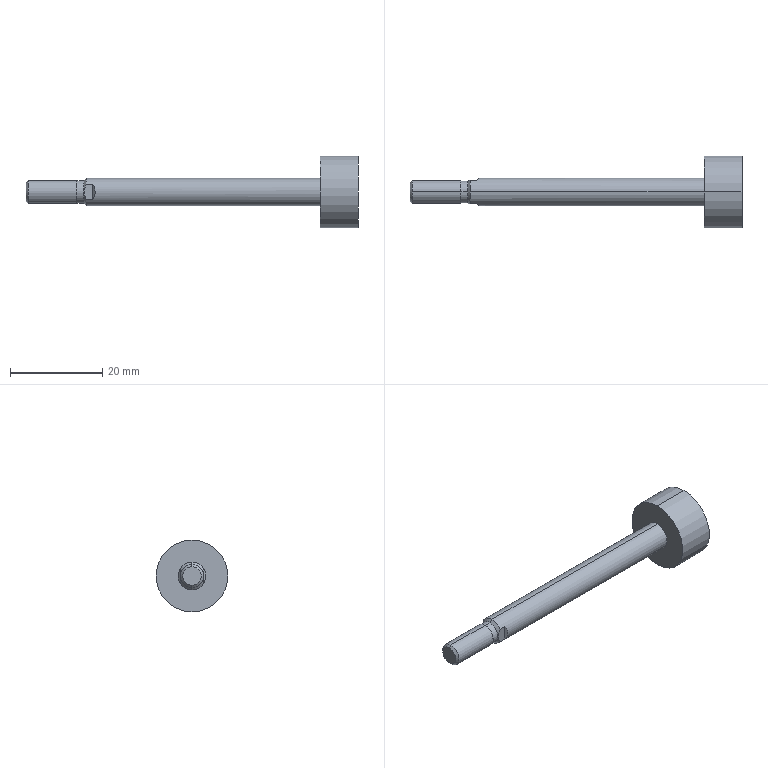Part | SolidWorks | features BaseBody 1 | 1 solid | 20 faces | box 72 x 15.6 x 15.6 mm | volume 3252 mm3 | plane 8 | cylinder 8 | cone 4 | commonest cylinder face diameters 4.8 x2 5 x2 6 x2 15.6 x2
STEP:
#1=CARTESIAN_POINT('',(-16.,0.,-2.01));
#2=VERTEX_POINT('',#1);
#3=CARTESIAN_POINT('',(-16.,0.,2.01));
#4=VERTEX_POINT('',#3);
#5=CARTESIAN_POINT('',(-16.,0.,0.));
#6=DIRECTION('',(1.,0.,0.));
#7=DIRECTION('',(0.,0.,-1.));
#8=AXIS2_PLACEMENT_3D('',#5,#6,#7);
#9=CIRCLE('',#8,2.01);
#10=EDGE_CURVE('',#2,#4,#9,.T.);
#11=ORIENTED_EDGE('',*,*,#10,.F.);
#12=CARTESIAN_POINT('',(-16.,0.,0.));
#13=DIRECTION('',(1.,0.,0.));
#14=DIRECTION('',(0.,0.,-1.));
#15=AXIS2_PLACEMENT_3D('',#12,#13,#14);
#16=CIRCLE('',#15,2.01);
#17=EDGE_CURVE('',#4,#2,#16,.T.);
#18=ORIENTED_EDGE('',*,*,#17,.F.);
#19=EDGE_LOOP('',(#11,#18));
#20=FACE_OUTER_BOUND('',#19,.T.);
#21=CARTESIAN_POINT('',(-16.,0.,0.));
#22=DIRECTION('',(1.,0.,0.));
#23=DIRECTION('',(0.,1.,0.));
#24=AXIS2_PLACEMENT_3D('',#21,#22,#23);
#25=PLANE('',#24);
#26=ADVANCED_FACE('',(#20),#25,.F.);
#27=CARTESIAN_POINT('',(-15.51,0.,2.5));
#28=VERTEX_POINT('',#27);
#29=CARTESIAN_POINT('',(-15.51,0.,2.5));
#30=DIRECTION('',(0.7071,0.,0.7071));
#31=VECTOR('',#30,1000.);
#32=LINE('',#29,#31);
#33=EDGE_CURVE('',#4,#28,#32,.T.);
#34=ORIENTED_EDGE('',*,*,#33,.F.);
#35=ORIENTED_EDGE('',*,*,#17,.T.);
#36=CARTESIAN_POINT('',(-15.51,0.,-2.5));
#37=VERTEX_POINT('',#36);
#38=CARTESIAN_POINT('',(-15.51,0.,-2.5));
#39=DIRECTION('',(0.7071,0.,-0.7071));
#40=VECTOR('',#39,1000.);
#41=LINE('',#38,#40);
#42=EDGE_CURVE('',#2,#37,#41,.T.);
#43=ORIENTED_EDGE('',*,*,#42,.T.);
#44=CARTESIAN_POINT('',(-15.51,0.,0.));
#45=DIRECTION('',(1.,0.,0.));
#46=DIRECTION('',(0.,0.,1.));
#47=AXIS2_PLACEMENT_3D('',#44,#45,#46);
#48=CIRCLE('',#47,2.5);
#49=EDGE_CURVE('',#28,#37,#48,.T.);
#50=ORIENTED_EDGE('',*,*,#49,.F.);
#51=EDGE_LOOP('',(#34,#35,#43,#50));
#52=FACE_OUTER_BOUND('',#51,.T.);
#53=CARTESIAN_POINT('',(-15.51,0.,0.));
#54=DIRECTION('',(1.,0.,0.));
#55=DIRECTION('',(0.,0.,-1.));
#56=AXIS2_PLACEMENT_3D('',#53,#54,#55);
#57=CONICAL_SURFACE('',#56,2.5,0.7854);
#58=ADVANCED_FACE('',(#52),#57,.T.);
#59=CARTESIAN_POINT('',(-5.,0.,-2.5));
#60=VERTEX_POINT('',#59);
#61=CARTESIAN_POINT('',(56.,0.,-2.5));
#62=DIRECTION('',(-1.,0.,0.));
#63=VECTOR('',#62,1000.);
#64=LINE('',#61,#63);
#65=EDGE_CURVE('',#60,#37,#64,.T.);
#66=ORIENTED_EDGE('',*,*,#65,.F.);
#67=CARTESIAN_POINT('',(-5.,0.,2.5));
#68=VERTEX_POINT('',#67);
#69=CARTESIAN_POINT('',(-5.,0.,0.));
#70=DIRECTION('',(-1.,0.,0.));
#71=DIRECTION('',(0.,0.,1.));
#72=AXIS2_PLACEMENT_3D('',#69,#70,#71);
#73=CIRCLE('',#72,2.5);
#74=EDGE_CURVE('',#60,#68,#73,.T.);
#75=ORIENTED_EDGE('',*,*,#74,.T.);
#76=CARTESIAN_POINT('',(56.,0.,2.5));
#77=DIRECTION('',(-1.,0.,0.));
#78=VECTOR('',#77,1000.);
#79=LINE('',#76,#78);
#80=EDGE_CURVE('',#68,#28,#79,.T.);
#81=ORIENTED_EDGE('',*,*,#80,.T.);
#82=ORIENTED_EDGE('',*,*,#49,.T.);
#83=EDGE_LOOP('',(#66,#75,#81,#82));
#84=FACE_OUTER_BOUND('',#83,.T.);
#85=CARTESIAN_POINT('',(56.,0.,0.));
#86=DIRECTION('',(-1.,0.,0.));
#87=DIRECTION('',(0.,0.,1.));
#88=AXIS2_PLACEMENT_3D('',#85,#86,#87);
#89=CYLINDRICAL_SURFACE('',#88,2.5);
#90=ADVANCED_FACE('',(#84),#89,.T.);
#91=CARTESIAN_POINT('',(56.,0.,7.8));
#92=VERTEX_POINT('',#91);
#93=CARTESIAN_POINT('',(56.,0.,-7.8));
#94=VERTEX_POINT('',#93);
#95=CARTESIAN_POINT('',(56.,0.,0.));
#96=DIRECTION('',(-1.,0.,0.));
#97=DIRECTION('',(0.,0.,1.));
#98=AXIS2_PLACEMENT_3D('',#95,#96,#97);
#99=CIRCLE('',#98,7.8);
#100=EDGE_CURVE('',#92,#94,#99,.T.);
#101=ORIENTED_EDGE('',*,*,#100,.F.);
#102=CARTESIAN_POINT('',(56.,0.,0.));
#103=DIRECTION('',(-1.,0.,0.));
#104=DIRECTION('',(0.,0.,1.));
#105=AXIS2_PLACEMENT_3D('',#102,#103,#104);
#106=CIRCLE('',#105,7.8);
#107=EDGE_CURVE('',#94,#92,#106,.T.);
#108=ORIENTED_EDGE('',*,*,#107,.F.);
#109=EDGE_LOOP('',(#101,#108));
#110=FACE_OUTER_BOUND('',#109,.T.);
#111=CARTESIAN_POINT('',(56.,7.8,0.));
#112=DIRECTION('',(-1.,0.,0.));
#113=DIRECTION('',(0.,0.,1.));
#114=AXIS2_PLACEMENT_3D('',#111,#112,#113);
#115=PLANE('',#114);
#116=ADVANCED_FACE('',(#110),#115,.F.);
#117=CARTESIAN_POINT('',(-5.,0.,2.4));
#118=VERTEX_POINT('',#117);
#119=CARTESIAN_POINT('',(-5.,0.,-2.4));
#120=VERTEX_POINT('',#119);
#121=CARTESIAN_POINT('',(-5.,0.,0.));
#122=DIRECTION('',(1.,0.,0.));
#123=DIRECTION('',(0.,0.,1.));
#124=AXIS2_PLACEMENT_3D('',#121,#122,#123);
#125=CIRCLE('',#124,2.4);
#126=EDGE_CURVE('',#118,#120,#125,.T.);
#127=ORIENTED_EDGE('',*,*,#126,.F.);
#128=CARTESIAN_POINT('',(-5.,0.,0.));
#129=DIRECTION('',(1.,0.,0.));
#130=DIRECTION('',(0.,0.,1.));
#131=AXIS2_PLACEMENT_3D('',#128,#129,#130);
#132=CIRCLE('',#131,2.4);
#133=EDGE_CURVE('',#120,#118,#132,.T.);
#134=ORIENTED_EDGE('',*,*,#133,.F.);
#135=EDGE_LOOP('',(#127,#134));
#136=FACE_BOUND('',#135,.T.);
#137=CARTESIAN_POINT('',(-5.,0.,0.));
#138=DIRECTION('',(-1.,0.,0.));
#139=DIRECTION('',(0.,0.,1.));
#140=AXIS2_PLACEMENT_3D('',#137,#138,#139);
#141=CIRCLE('',#140,2.5);
#142=EDGE_CURVE('',#68,#60,#141,.T.);
#143=ORIENTED_EDGE('',*,*,#142,.F.);
#144=ORIENTED_EDGE('',*,*,#74,.F.);
#145=EDGE_LOOP('',(#143,#144));
#146=FACE_OUTER_BOUND('',#145,.T.);
#147=CARTESIAN_POINT('',(-5.,2.5,0.));
#148=DIRECTION('',(-1.,0.,0.));
#149=DIRECTION('',(0.,0.,1.));
#150=AXIS2_PLACEMENT_3D('',#147,#148,#149);
#151=PLANE('',#150);
#152=ADVANCED_FACE('',(#136,#146),#151,.F.);
#153=CARTESIAN_POINT('',(47.8,0.,-7.8));
#154=VERTEX_POINT('',#153);
#155=CARTESIAN_POINT('',(56.,0.,-7.8));
#156=DIRECTION('',(-1.,0.,0.));
#157=VECTOR('',#156,1000.);
#158=LINE('',#155,#157);
#159=EDGE_CURVE('',#94,#154,#158,.T.);
#160=ORIENTED_EDGE('',*,*,#159,.F.);
#161=ORIENTED_EDGE('',*,*,#107,.T.);
#162=CARTESIAN_POINT('',(47.8,0.,7.8));
#163=VERTEX_POINT('',#162);
#164=CARTESIAN_POINT('',(56.,0.,7.8));
#165=DIRECTION('',(-1.,0.,0.));
#166=VECTOR('',#165,1000.);
#167=LINE('',#164,#166);
#168=EDGE_CURVE('',#92,#163,#167,.T.);
#169=ORIENTED_EDGE('',*,*,#168,.T.);
#170=CARTESIAN_POINT('',(47.8,0.,0.));
#171=DIRECTION('',(1.,0.,0.));
#172=DIRECTION('',(0.,0.,1.));
#173=AXIS2_PLACEMENT_3D('',#170,#171,#172);
#174=CIRCLE('',#173,7.8);
#175=EDGE_CURVE('',#163,#154,#174,.T.);
#176=ORIENTED_EDGE('',*,*,#175,.T.);
#177=EDGE_LOOP('',(#160,#161,#169,#176));
#178=FACE_OUTER_BOUND('',#177,.T.);
#179=CARTESIAN_POINT('',(56.,0.,0.));
#180=DIRECTION('',(-1.,0.,0.));
#181=DIRECTION('',(0.,0.,1.));
#182=AXIS2_PLACEMENT_3D('',#179,#180,#181);
#183=CYLINDRICAL_SURFACE('',#182,7.8);
#184=ADVANCED_FACE('',(#178),#183,.T.);
#185=CARTESIAN_POINT('',(-1.5,2.5,-1.658));
#186=VERTEX_POINT('',#185);
#187=CARTESIAN_POINT('',(-2.9,2.5,-1.658));
#188=VERTEX_POINT('',#187);
#189=CARTESIAN_POINT('',(-18.5,2.5,-1.658));
#190=DIRECTION('',(-1.,0.,0.));
#191=VECTOR('',#190,1000.);
#192=LINE('',#189,#191);
#193=EDGE_CURVE('',#186,#188,#192,.T.);
#194=ORIENTED_EDGE('',*,*,#193,.T.);
#195=CARTESIAN_POINT('',(-2.9,2.5,1.658));
#196=VERTEX_POINT('',#195);
#197=CARTESIAN_POINT('',(-2.9,2.5,1.658));
#198=CARTESIAN_POINT('',(-2.976,2.5,1.52));
#199=CARTESIAN_POINT('',(-3.044,2.5,1.385));
#200=CARTESIAN_POINT('',(-3.133,2.5,1.187));
#201=CARTESIAN_POINT('',(-3.161,2.5,1.121));
#202=CARTESIAN_POINT('',(-3.199,2.5,1.024));
#203=CARTESIAN_POINT('',(-3.217,2.5,0.9749));
#204=CARTESIAN_POINT('',(-3.234,2.5,0.9264));
#205=CARTESIAN_POINT('',(-3.245,2.5,0.8941));
#206=CARTESIAN_POINT('',(-3.25,2.5,0.8796));
#207=CARTESIAN_POINT('',(-3.279,2.5,0.7907));
#208=CARTESIAN_POINT('',(-3.299,2.5,0.7199));
#209=CARTESIAN_POINT('',(-3.326,2.5,0.6139));
#210=CARTESIAN_POINT('',(-3.334,2.5,0.5785));
#211=CARTESIAN_POINT('',(-3.349,2.5,0.5078));
#212=CARTESIAN_POINT('',(-3.356,2.5,0.4737));
#213=CARTESIAN_POINT('',(-3.387,2.5,0.2894));
#214=CARTESIAN_POINT('',(-3.4,2.5,0.1457));
#215=CARTESIAN_POINT('',(-3.4,2.5,-0.1432));
#216=CARTESIAN_POINT('',(-3.388,2.5,-0.2845));
#217=CARTESIAN_POINT('',(-3.352,2.5,-0.4978));
#218=CARTESIAN_POINT('',(-3.337,2.5,-0.5692));
#219=CARTESIAN_POINT('',(-3.31,2.5,-0.6771));
#220=CARTESIAN_POINT('',(-3.296,2.5,-0.7314));
#221=CARTESIAN_POINT('',(-3.277,2.5,-0.7952));
#222=CARTESIAN_POINT('',(-3.268,2.5,-0.8227));
#223=CARTESIAN_POINT('',(-3.262,2.5,-0.8411));
#224=CARTESIAN_POINT('',(-3.259,2.5,-0.8514));
#225=CARTESIAN_POINT('',(-3.172,2.5,-1.118));
#226=CARTESIAN_POINT('',(-3.053,2.5,-1.381));
#227=CARTESIAN_POINT('',(-2.9,2.5,-1.658));
#228=B_SPLINE_CURVE_WITH_KNOTS('',3,(#197,#198,#199,#200,#201,#202,#203,#204,#205,#206,#207,#208,#209,#210,#211,#212,#213,#214,#215,#216,#217,#218,#219,#220,#221,#222,#223,#224,#225,#226,#227),.UNSPECIFIED.,.F.,.F.,(4,2,2,1,2,2,2,2,2,2,2,2,1,1,2,2,4),(0.,0.125,0.1875,0.2187,0.2344,0.25,0.3125,0.3437,0.375,0.5,0.625,0.6875,0.7187,0.7344,0.7422,0.75,1.),.UNSPECIFIED.);
#229=EDGE_CURVE('',#196,#188,#228,.T.);
#230=ORIENTED_EDGE('',*,*,#229,.F.);
#231=CARTESIAN_POINT('',(-1.5,2.5,1.658));
#232=VERTEX_POINT('',#231);
#233=CARTESIAN_POINT('',(-18.5,2.5,1.658));
#234=DIRECTION('',(1.,0.,0.));
#235=VECTOR('',#234,1000.);
#236=LINE('',#233,#235);
#237=EDGE_CURVE('',#196,#232,#236,.T.);
#238=ORIENTED_EDGE('',*,*,#237,.T.);
#239=CARTESIAN_POINT('',(-1.5,2.5,6.));
#240=DIRECTION('',(0.,0.,1.));
#241=VECTOR('',#240,1000.);
#242=LINE('',#239,#241);
#243=EDGE_CURVE('',#186,#232,#242,.T.);
#244=ORIENTED_EDGE('',*,*,#243,.F.);
#245=EDGE_LOOP('',(#194,#230,#238,#244));
#246=FACE_OUTER_BOUND('',#245,.T.);
#247=CARTESIAN_POINT('',(-18.5,2.5,6.));
#248=DIRECTION('',(0.,1.,0.));
#249=DIRECTION('',(1.,0.,0.));
#250=AXIS2_PLACEMENT_3D('',#247,#248,#249);
#251=PLANE('',#250);
#252=ADVANCED_FACE('',(#246),#251,.T.);
#253=CARTESIAN_POINT('',(-1.5,-2.5,1.658));
#254=VERTEX_POINT('',#253);
#255=CARTESIAN_POINT('',(-2.9,-2.5,1.658));
#256=VERTEX_POINT('',#255);
#257=CARTESIAN_POINT('',(-1.5,-2.5,1.658));
#258=DIRECTION('',(-1.,0.,0.));
#259=VECTOR('',#258,1000.);
#260=LINE('',#257,#259);
#261=EDGE_CURVE('',#254,#256,#260,.T.);
#262=ORIENTED_EDGE('',*,*,#261,.T.);
#263=CARTESIAN_POINT('',(-2.9,-2.5,-1.658));
#264=VERTEX_POINT('',#263);
#265=CARTESIAN_POINT('',(-2.9,-2.5,-1.658));
#266=CARTESIAN_POINT('',(-2.976,-2.5,-1.52));
#267=CARTESIAN_POINT('',(-3.044,-2.5,-1.385));
#268=CARTESIAN_POINT('',(-3.133,-2.5,-1.187));
#269=CARTESIAN_POINT('',(-3.161,-2.5,-1.121));
#270=CARTESIAN_POINT('',(-3.199,-2.5,-1.024));
#271=CARTESIAN_POINT('',(-3.217,-2.5,-0.9749));
#272=CARTESIAN_POINT('',(-3.234,-2.5,-0.9264));
#273=CARTESIAN_POINT('',(-3.245,-2.5,-0.8941));
#274=CARTESIAN_POINT('',(-3.25,-2.5,-0.8796));
#275=CARTESIAN_POINT('',(-3.279,-2.5,-0.7907));
#276=CARTESIAN_POINT('',(-3.299,-2.5,-0.7199));
#277=CARTESIAN_POINT('',(-3.326,-2.5,-0.6139));
#278=CARTESIAN_POINT('',(-3.334,-2.5,-0.5785));
#279=CARTESIAN_POINT('',(-3.349,-2.5,-0.5078));
#280=CARTESIAN_POINT('',(-3.356,-2.5,-0.4737));
#281=CARTESIAN_POINT('',(-3.387,-2.5,-0.2894));
#282=CARTESIAN_POINT('',(-3.4,-2.5,-0.1457));
#283=CARTESIAN_POINT('',(-3.4,-2.5,0.1432));
#284=CARTESIAN_POINT('',(-3.388,-2.5,0.2845));
#285=CARTESIAN_POINT('',(-3.352,-2.5,0.4978));
#286=CARTESIAN_POINT('',(-3.337,-2.5,0.5692));
#287=CARTESIAN_POINT('',(-3.31,-2.5,0.6771));
#288=CARTESIAN_POINT('',(-3.296,-2.5,0.7314));
#289=CARTESIAN_POINT('',(-3.277,-2.5,0.7952));
#290=CARTESIAN_POINT('',(-3.268,-2.5,0.8227));
#291=CARTESIAN_POINT('',(-3.262,-2.5,0.8411));
#292=CARTESIAN_POINT('',(-3.259,-2.5,0.8514));
#293=CARTESIAN_POINT('',(-3.172,-2.5,1.118));
#294=CARTESIAN_POINT('',(-3.053,-2.5,1.381));
#295=CARTESIAN_POINT('',(-2.9,-2.5,1.658));
#296=B_SPLINE_CURVE_WITH_KNOTS('',3,(#265,#266,#267,#268,#269,#270,#271,#272,#273,#274,#275,#276,#277,#278,#279,#280,#281,#282,#283,#284,#285,#286,#287,#288,#289,#290,#291,#292,#293,#294,#295),.UNSPECIFIED.,.F.,.F.,(4,2,2,1,2,2,2,2,2,2,2,2,1,1,2,2,4),(0.,0.125,0.1875,0.2187,0.2344,0.25,0.3125,0.3438,0.375,0.5,0.625,0.6875,0.7188,0.7344,0.7422,0.75,1.),.UNSPECIFIED.);
#297=EDGE_CURVE('',#264,#256,#296,.T.);
#298=ORIENTED_EDGE('',*,*,#297,.F.);
#299=CARTESIAN_POINT('',(-1.5,-2.5,-1.658));
#300=VERTEX_POINT('',#299);
#301=CARTESIAN_POINT('',(-1.5,-2.5,-1.658));
#302=DIRECTION('',(1.,0.,0.));
#303=VECTOR('',#302,1000.);
#304=LINE('',#301,#303);
#305=EDGE_CURVE('',#264,#300,#304,.T.);
#306=ORIENTED_EDGE('',*,*,#305,.T.);
#307=CARTESIAN_POINT('',(-1.5,-2.5,6.));
#308=DIRECTION('',(0.,0.,-1.));
#309=VECTOR('',#308,1000.);
#310=LINE('',#307,#309);
#311=EDGE_CURVE('',#254,#300,#310,.T.);
#312=ORIENTED_EDGE('',*,*,#311,.F.);
#313=EDGE_LOOP('',(#262,#298,#306,#312));
#314=FACE_OUTER_BOUND('',#313,.T.);
#315=CARTESIAN_POINT('',(-1.5,-2.5,6.));
#316=DIRECTION('',(0.,-1.,0.));
#317=DIRECTION('',(0.,0.,-1.));
#318=AXIS2_PLACEMENT_3D('',#315,#316,#317);
#319=PLANE('',#318);
#320=ADVANCED_FACE('',(#314),#319,.T.);
#321=CARTESIAN_POINT('',(-3.5,0.,-2.4));
#322=VERTEX_POINT('',#321);
#323=CARTESIAN_POINT('',(56.,0.,-2.4));
#324=DIRECTION('',(-1.,0.,0.));
#325=VECTOR('',#324,1000.);
#326=LINE('',#323,#325);
#327=EDGE_CURVE('',#322,#120,#326,.T.);
#328=ORIENTED_EDGE('',*,*,#327,.F.);
#329=CARTESIAN_POINT('',(-3.5,0.,2.4));
#330=VERTEX_POINT('',#329);
#331=CARTESIAN_POINT('',(-3.5,0.,0.));
#332=DIRECTION('',(1.,0.,0.));
#333=DIRECTION('',(0.,0.,-1.));
#334=AXIS2_PLACEMENT_3D('',#331,#332,#333);
#335=CIRCLE('',#334,2.4);
#336=EDGE_CURVE('',#330,#322,#335,.T.);
#337=ORIENTED_EDGE('',*,*,#336,.F.);
#338=CARTESIAN_POINT('',(56.,0.,2.4));
#339=DIRECTION('',(-1.,0.,0.));
#340=VECTOR('',#339,1000.);
#341=LINE('',#338,#340);
#342=EDGE_CURVE('',#330,#118,#341,.T.);
#343=ORIENTED_EDGE('',*,*,#342,.T.);
#344=ORIENTED_EDGE('',*,*,#126,.T.);
#345=EDGE_LOOP('',(#328,#337,#343,#344));
#346=FACE_OUTER_BOUND('',#345,.T.);
#347=CARTESIAN_POINT('',(56.,0.,0.));
#348=DIRECTION('',(-1.,0.,0.));
#349=DIRECTION('',(0.,0.,1.));
#350=AXIS2_PLACEMENT_3D('',#347,#348,#349);
#351=CYLINDRICAL_SURFACE('',#350,2.4);
#352=ADVANCED_FACE('',(#346),#351,.T.);
#353=CARTESIAN_POINT('',(47.8,0.,3.));
#354=VERTEX_POINT('',#353);
#355=CARTESIAN_POINT('',(47.8,0.,-3.));
#356=VERTEX_POINT('',#355);
#357=CARTESIAN_POINT('',(47.8,0.,0.));
#358=DIRECTION('',(-1.,0.,0.));
#359=DIRECTION('',(0.,0.,1.));
#360=AXIS2_PLACEMENT_3D('',#357,#358,#359);
#361=CIRCLE('',#360,3.);
#362=EDGE_CURVE('',#354,#356,#361,.T.);
#363=ORIENTED_EDGE('',*,*,#362,.F.);
#364=CARTESIAN_POINT('',(47.8,0.,0.));
#365=DIRECTION('',(-1.,0.,0.));
#366=DIRECTION('',(0.,0.,1.));
#367=AXIS2_PLACEMENT_3D('',#364,#365,#366);
#368=CIRCLE('',#367,3.);
#369=EDGE_CURVE('',#356,#354,#368,.T.);
#370=ORIENTED_EDGE('',*,*,#369,.F.);
#371=EDGE_LOOP('',(#363,#370));
#372=FACE_BOUND('',#371,.T.);
#373=ORIENTED_EDGE('',*,*,#175,.F.);
#374=CARTESIAN_POINT('',(47.8,0.,0.));
#375=DIRECTION('',(1.,0.,0.));
#376=DIRECTION('',(0.,0.,1.));
#377=AXIS2_PLACEMENT_3D('',#374,#375,#376);
#378=CIRCLE('',#377,7.8);
#379=EDGE_CURVE('',#154,#163,#378,.T.);
#380=ORIENTED_EDGE('',*,*,#379,.F.);
#381=EDGE_LOOP('',(#373,#380));
#382=FACE_OUTER_BOUND('',#381,.T.);
#383=CARTESIAN_POINT('',(47.8,3.,0.));
#384=DIRECTION('',(1.,0.,0.));
#385=DIRECTION('',(0.,1.,0.));
#386=AXIS2_PLACEMENT_3D('',#383,#384,#385);
#387=PLANE('',#386);
#388=ADVANCED_FACE('',(#372,#382),#387,.F.);
#389=CARTESIAN_POINT('',(-1.5,-2.5,1.658));
#390=CARTESIAN_POINT('',(-0.8125,-3.188,0.6219));
#391=CARTESIAN_POINT('',(-0.8125,-3.188,-0.6219));
#392=CARTESIAN_POINT('',(-1.5,-2.5,-1.658));
#393=(BOUNDED_CURVE()B_SPLINE_CURVE(3,(#389,#390,#391,#392),.UNSPECIFIED.,.F.,.F.)B_SPLINE_CURVE_WITH_KNOTS((4,4),(2.556,3.727),.UNSPECIFIED.)CURVE()GEOMETRIC_REPRESENTATION_ITEM()RATIONAL_B_SPLINE_CURVE((1.,0.8889,0.8889,1.))REPRESENTATION_ITEM(''));
#394=EDGE_CURVE('',#254,#300,#393,.T.);
#395=ORIENTED_EDGE('',*,*,#394,.F.);
#396=ORIENTED_EDGE('',*,*,#311,.T.);
#397=EDGE_LOOP('',(#395,#396));
#398=FACE_OUTER_BOUND('',#397,.T.);
#399=CARTESIAN_POINT('',(-1.,-3.,6.));
#400=DIRECTION('',(-0.7071,-0.7071,0.));
#401=DIRECTION('',(-0.7071,0.7071,0.));
#402=AXIS2_PLACEMENT_3D('',#399,#400,#401);
#403=PLANE('',#402);
#404=ADVANCED_FACE('',(#398),#403,.T.);
#405=CARTESIAN_POINT('',(-1.5,2.5,-1.658));
#406=CARTESIAN_POINT('',(-0.8125,3.188,-0.6219));
#407=CARTESIAN_POINT('',(-0.8125,3.188,0.6219));
#408=CARTESIAN_POINT('',(-1.5,2.5,1.658));
#409=(BOUNDED_CURVE()B_SPLINE_CURVE(3,(#405,#406,#407,#408),.UNSPECIFIED.,.F.,.F.)B_SPLINE_CURVE_WITH_KNOTS((4,4),(2.556,3.727),.UNSPECIFIED.)CURVE()GEOMETRIC_REPRESENTATION_ITEM()RATIONAL_B_SPLINE_CURVE((1.,0.8889,0.8889,1.))REPRESENTATION_ITEM(''));
#410=EDGE_CURVE('',#186,#232,#409,.T.);
#411=ORIENTED_EDGE('',*,*,#410,.F.);
#412=ORIENTED_EDGE('',*,*,#243,.T.);
#413=EDGE_LOOP('',(#411,#412));
#414=FACE_OUTER_BOUND('',#413,.T.);
#415=CARTESIAN_POINT('',(-1.5,2.5,6.));
#416=DIRECTION('',(-0.7071,0.7071,0.));
#417=DIRECTION('',(0.,0.,1.));
#418=AXIS2_PLACEMENT_3D('',#415,#416,#417);
#419=PLANE('',#418);
#420=ADVANCED_FACE('',(#414),#419,.T.);
#421=CARTESIAN_POINT('',(-2.9,0.,3.));
#422=VERTEX_POINT('',#421);
#423=CARTESIAN_POINT('',(-2.9,0.,3.));
#424=DIRECTION('',(0.7071,0.,0.7071));
#425=VECTOR('',#424,1000.);
#426=LINE('',#423,#425);
#427=EDGE_CURVE('',#330,#422,#426,.T.);
#428=ORIENTED_EDGE('',*,*,#427,.F.);
#429=ORIENTED_EDGE('',*,*,#336,.T.);
#430=CARTESIAN_POINT('',(-2.9,0.,-3.));
#431=VERTEX_POINT('',#430);
#432=CARTESIAN_POINT('',(-2.9,0.,-3.));
#433=DIRECTION('',(0.7071,0.,-0.7071));
#434=VECTOR('',#433,1000.);
#435=LINE('',#432,#434);
#436=EDGE_CURVE('',#322,#431,#435,.T.);
#437=ORIENTED_EDGE('',*,*,#436,.T.);
#438=CARTESIAN_POINT('',(-2.9,0.,0.));
#439=DIRECTION('',(1.,0.,0.));
#440=DIRECTION('',(0.,0.,1.));
#441=AXIS2_PLACEMENT_3D('',#438,#439,#440);
#442=CIRCLE('',#441,3.);
#443=EDGE_CURVE('',#264,#431,#442,.T.);
#444=ORIENTED_EDGE('',*,*,#443,.F.);
#445=ORIENTED_EDGE('',*,*,#297,.T.);
#446=CARTESIAN_POINT('',(-2.9,0.,0.));
#447=DIRECTION('',(1.,0.,0.));
#448=DIRECTION('',(0.,0.,1.));
#449=AXIS2_PLACEMENT_3D('',#446,#447,#448);
#450=CIRCLE('',#449,3.);
#451=EDGE_CURVE('',#422,#256,#450,.T.);
#452=ORIENTED_EDGE('',*,*,#451,.F.);
#453=EDGE_LOOP('',(#428,#429,#437,#444,#445,#452));
#454=FACE_OUTER_BOUND('',#453,.T.);
#455=CARTESIAN_POINT('',(-2.9,0.,0.));
#456=DIRECTION('',(1.,0.,0.));
#457=DIRECTION('',(0.,0.,-1.));
#458=AXIS2_PLACEMENT_3D('',#455,#456,#457);
#459=CONICAL_SURFACE('',#458,3.,0.7854);
#460=ADVANCED_FACE('',(#454),#459,.T.);
#461=CARTESIAN_POINT('',(56.,0.,-3.));
#462=DIRECTION('',(-1.,0.,0.));
#463=VECTOR('',#462,1000.);
#464=LINE('',#461,#463);
#465=EDGE_CURVE('',#356,#431,#464,.T.);
#466=ORIENTED_EDGE('',*,*,#465,.F.);
#467=ORIENTED_EDGE('',*,*,#369,.T.);
#468=CARTESIAN_POINT('',(56.,0.,3.));
#469=DIRECTION('',(-1.,0.,0.));
#470=VECTOR('',#469,1000.);
#471=LINE('',#468,#470);
#472=EDGE_CURVE('',#354,#422,#471,.T.);
#473=ORIENTED_EDGE('',*,*,#472,.T.);
#474=ORIENTED_EDGE('',*,*,#451,.T.);
#475=ORIENTED_EDGE('',*,*,#261,.F.);
#476=ORIENTED_EDGE('',*,*,#394,.T.);
#477=ORIENTED_EDGE('',*,*,#305,.F.);
#478=ORIENTED_EDGE('',*,*,#443,.T.);
#479=EDGE_LOOP('',(#466,#467,#473,#474,#475,#476,#477,#478));
#480=FACE_OUTER_BOUND('',#479,.T.);
#481=CARTESIAN_POINT('',(56.,0.,0.));
#482=DIRECTION('',(-1.,0.,0.));
#483=DIRECTION('',(0.,0.,1.));
#484=AXIS2_PLACEMENT_3D('',#481,#482,#483);
#485=CYLINDRICAL_SURFACE('',#484,3.);
#486=ADVANCED_FACE('',(#480),#485,.T.);
#487=ORIENTED_EDGE('',*,*,#10,.T.);
#488=ORIENTED_EDGE('',*,*,#33,.T.);
#489=CARTESIAN_POINT('',(-15.51,0.,0.));
#490=DIRECTION('',(1.,0.,0.));
#491=DIRECTION('',(0.,0.,1.));
#492=AXIS2_PLACEMENT_3D('',#489,#490,#491);
#493=CIRCLE('',#492,2.5);
#494=EDGE_CURVE('',#37,#28,#493,.T.);
#495=ORIENTED_EDGE('',*,*,#494,.F.);
#496=ORIENTED_EDGE('',*,*,#42,.F.);
#497=EDGE_LOOP('',(#487,#488,#495,#496));
#498=FACE_OUTER_BOUND('',#497,.T.);
#499=CARTESIAN_POINT('',(-15.51,0.,0.));
#500=DIRECTION('',(1.,0.,0.));
#501=DIRECTION('',(0.,0.,-1.));
#502=AXIS2_PLACEMENT_3D('',#499,#500,#501);
#503=CONICAL_SURFACE('',#502,2.5,0.7854);
#504=ADVANCED_FACE('',(#498),#503,.T.);
#505=ORIENTED_EDGE('',*,*,#142,.T.);
#506=ORIENTED_EDGE('',*,*,#65,.T.);
#507=ORIENTED_EDGE('',*,*,#494,.T.);
#508=ORIENTED_EDGE('',*,*,#80,.F.);
#509=EDGE_LOOP('',(#505,#506,#507,#508));
#510=FACE_OUTER_BOUND('',#509,.T.);
#511=CARTESIAN_POINT('',(56.,0.,0.));
#512=DIRECTION('',(-1.,0.,0.));
#513=DIRECTION('',(0.,0.,1.));
#514=AXIS2_PLACEMENT_3D('',#511,#512,#513);
#515=CYLINDRICAL_SURFACE('',#514,2.5);
#516=ADVANCED_FACE('',(#510),#515,.T.);
#517=ORIENTED_EDGE('',*,*,#100,.T.);
#518=ORIENTED_EDGE('',*,*,#159,.T.);
#519=ORIENTED_EDGE('',*,*,#379,.T.);
#520=ORIENTED_EDGE('',*,*,#168,.F.);
#521=EDGE_LOOP('',(#517,#518,#519,#520));
#522=FACE_OUTER_BOUND('',#521,.T.);
#523=CARTESIAN_POINT('',(56.,0.,0.));
#524=DIRECTION('',(-1.,0.,0.));
#525=DIRECTION('',(0.,0.,1.));
#526=AXIS2_PLACEMENT_3D('',#523,#524,#525);
#527=CYLINDRICAL_SURFACE('',#526,7.8);
#528=ADVANCED_FACE('',(#522),#527,.T.);
#529=CARTESIAN_POINT('',(-3.5,0.,0.));
#530=DIRECTION('',(1.,0.,0.));
#531=DIRECTION('',(0.,0.,-1.));
#532=AXIS2_PLACEMENT_3D('',#529,#530,#531);
#533=CIRCLE('',#532,2.4);
#534=EDGE_CURVE('',#322,#330,#533,.T.);
#535=ORIENTED_EDGE('',*,*,#534,.F.);
#536=ORIENTED_EDGE('',*,*,#327,.T.);
#537=ORIENTED_EDGE('',*,*,#133,.T.);
#538=ORIENTED_EDGE('',*,*,#342,.F.);
#539=EDGE_LOOP('',(#535,#536,#537,#538));
#540=FACE_OUTER_BOUND('',#539,.T.);
#541=CARTESIAN_POINT('',(56.,0.,0.));
#542=DIRECTION('',(-1.,0.,0.));
#543=DIRECTION('',(0.,0.,1.));
#544=AXIS2_PLACEMENT_3D('',#541,#542,#543);
#545=CYLINDRICAL_SURFACE('',#544,2.4);
#546=ADVANCED_FACE('',(#540),#545,.T.);
#547=ORIENTED_EDGE('',*,*,#534,.T.);
#548=ORIENTED_EDGE('',*,*,#427,.T.);
#549=CARTESIAN_POINT('',(-2.9,0.,0.));
#550=DIRECTION('',(1.,0.,0.));
#551=DIRECTION('',(0.,0.,1.));
#552=AXIS2_PLACEMENT_3D('',#549,#550,#551);
#553=CIRCLE('',#552,3.);
#554=EDGE_CURVE('',#196,#422,#553,.T.);
#555=ORIENTED_EDGE('',*,*,#554,.F.);
#556=ORIENTED_EDGE('',*,*,#229,.T.);
#557=CARTESIAN_POINT('',(-2.9,0.,0.));
#558=DIRECTION('',(1.,0.,0.));
#559=DIRECTION('',(0.,0.,1.));
#560=AXIS2_PLACEMENT_3D('',#557,#558,#559);
#561=CIRCLE('',#560,3.);
#562=EDGE_CURVE('',#431,#188,#561,.T.);
#563=ORIENTED_EDGE('',*,*,#562,.F.);
#564=ORIENTED_EDGE('',*,*,#436,.F.);
#565=EDGE_LOOP('',(#547,#548,#555,#556,#563,#564));
#566=FACE_OUTER_BOUND('',#565,.T.);
#567=CARTESIAN_POINT('',(-2.9,0.,0.));
#568=DIRECTION('',(1.,0.,0.));
#569=DIRECTION('',(0.,0.,-1.));
#570=AXIS2_PLACEMENT_3D('',#567,#568,#569);
#571=CONICAL_SURFACE('',#570,3.,0.7854);
#572=ADVANCED_FACE('',(#566),#571,.T.);
#573=ORIENTED_EDGE('',*,*,#362,.T.);
#574=ORIENTED_EDGE('',*,*,#465,.T.);
#575=ORIENTED_EDGE('',*,*,#562,.T.);
#576=ORIENTED_EDGE('',*,*,#193,.F.);
#577=ORIENTED_EDGE('',*,*,#410,.T.);
#578=ORIENTED_EDGE('',*,*,#237,.F.);
#579=ORIENTED_EDGE('',*,*,#554,.T.);
#580=ORIENTED_EDGE('',*,*,#472,.F.);
#581=EDGE_LOOP('',(#573,#574,#575,#576,#577,#578,#579,#580));
#582=FACE_OUTER_BOUND('',#581,.T.);
#583=CARTESIAN_POINT('',(56.,0.,0.));
#584=DIRECTION('',(-1.,0.,0.));
#585=DIRECTION('',(0.,0.,1.));
#586=AXIS2_PLACEMENT_3D('',#583,#584,#585);
#587=CYLINDRICAL_SURFACE('',#586,3.);
#588=ADVANCED_FACE('',(#582),#587,.T.);
#589=CLOSED_SHELL('',(#26,#58,#90,#116,#152,#184,#252,#320,#352,#388,#404,#420,#460,#486,#504,#516,#528,#546,#572,#588));
#590=MANIFOLD_SOLID_BREP('',#589);
#591=CARTESIAN_POINT('',(0.,0.,0.));
#592=DIRECTION('',(0.,0.,1.));
#593=DIRECTION('',(1.,0.,0.));
#594=AXIS2_PLACEMENT_3D('',#591,#592,#593);
#595=(LENGTH_UNIT()NAMED_UNIT(*)SI_UNIT(.MILLI.,.METRE.));
#596=UNCERTAINTY_MEASURE_WITH_UNIT(LENGTH_MEASURE(0.00001),#595,'','');
#597=(NAMED_UNIT(*)PLANE_ANGLE_UNIT()SI_UNIT($,.RADIAN.));
#598=(NAMED_UNIT(*)SI_UNIT($,.STERADIAN.)SOLID_ANGLE_UNIT());
#599=(GEOMETRIC_REPRESENTATION_CONTEXT(3)GLOBAL_UNCERTAINTY_ASSIGNED_CONTEXT((#596))GLOBAL_UNIT_ASSIGNED_CONTEXT((#595,#597,#598))REPRESENTATION_CONTEXT('',''));
#600=ADVANCED_BREP_SHAPE_REPRESENTATION('',(#590,#594),#599);